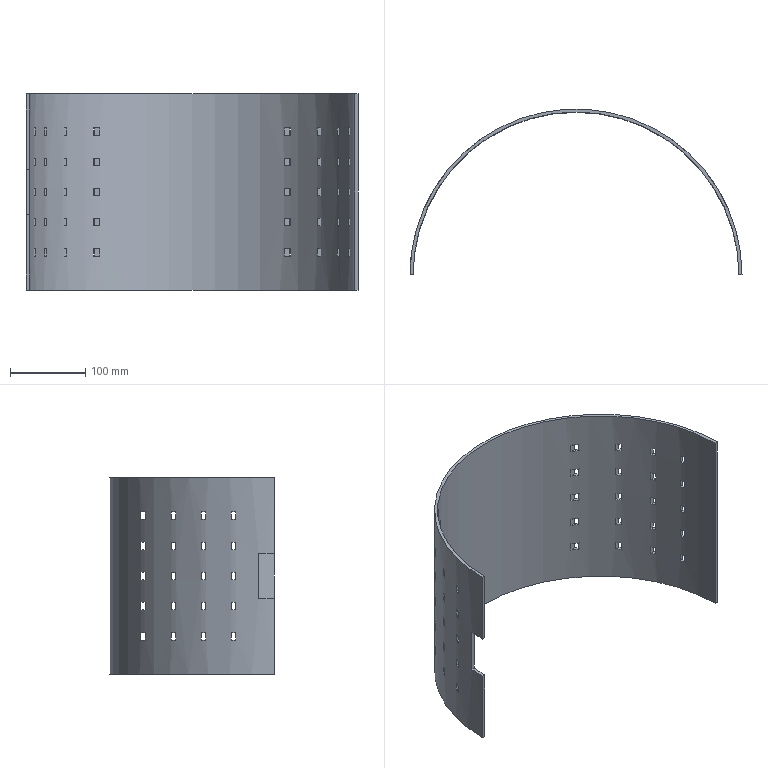Part | SolidWorks | features ICE 2, Extrusion 1 | 1 solid | 170 faces | box 439.995 x 219 x 260 mm | volume 692901 mm3 | plane 168 | cylinder 2 | commonest cylinder face diameters 432 x1 440 x1